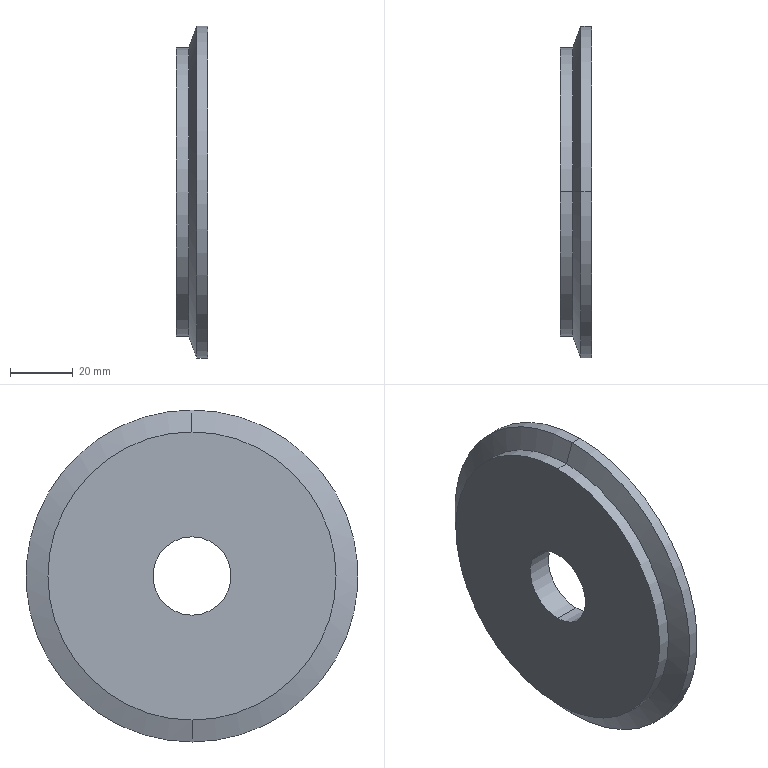Part | SolidWorks | features Revolution 1 | 1 solid | 13 faces | box 10 x 106 x 106 mm | volume 67420 mm3 | cylinder 8 | plane 3 | cone 2 | commonest cylinder face diameters 25 x2 62 x2 92 x2 106 x2
STEP:
#1=CARTESIAN_POINT('',(-7.771,0.,-46.));
#2=VERTEX_POINT('',#1);
#3=CARTESIAN_POINT('',(-7.771,0.,46.));
#4=VERTEX_POINT('',#3);
#5=CARTESIAN_POINT('',(-7.771,0.,0.));
#6=DIRECTION('',(1.,0.,0.));
#7=DIRECTION('',(0.,0.,-1.));
#8=AXIS2_PLACEMENT_3D('',#5,#6,#7);
#9=CIRCLE('',#8,46.);
#10=EDGE_CURVE('',#2,#4,#9,.T.);
#11=ORIENTED_EDGE('',*,*,#10,.T.);
#12=CARTESIAN_POINT('',(-5.271,0.,53.));
#13=VERTEX_POINT('',#12);
#14=CARTESIAN_POINT('',(-5.271,0.,53.));
#15=DIRECTION('',(0.3363,0.,0.9417));
#16=VECTOR('',#15,1000.);
#17=LINE('',#14,#16);
#18=EDGE_CURVE('',#4,#13,#17,.T.);
#19=ORIENTED_EDGE('',*,*,#18,.T.);
#20=CARTESIAN_POINT('',(-5.271,0.,-53.));
#21=VERTEX_POINT('',#20);
#22=CARTESIAN_POINT('',(-5.271,0.,0.));
#23=DIRECTION('',(1.,0.,0.));
#24=DIRECTION('',(0.,0.,-1.));
#25=AXIS2_PLACEMENT_3D('',#22,#23,#24);
#26=CIRCLE('',#25,53.);
#27=EDGE_CURVE('',#21,#13,#26,.T.);
#28=ORIENTED_EDGE('',*,*,#27,.F.);
#29=CARTESIAN_POINT('',(-5.271,0.,-53.));
#30=DIRECTION('',(0.3363,0.,-0.9417));
#31=VECTOR('',#30,1000.);
#32=LINE('',#29,#31);
#33=EDGE_CURVE('',#2,#21,#32,.T.);
#34=ORIENTED_EDGE('',*,*,#33,.F.);
#35=EDGE_LOOP('',(#11,#19,#28,#34));
#36=FACE_OUTER_BOUND('',#35,.T.);
#37=CARTESIAN_POINT('',(-5.271,0.,0.));
#38=DIRECTION('',(1.,0.,0.));
#39=DIRECTION('',(0.,0.,-1.));
#40=AXIS2_PLACEMENT_3D('',#37,#38,#39);
#41=CONICAL_SURFACE('',#40,53.,1.228);
#42=ADVANCED_FACE('',(#36),#41,.T.);
#43=ORIENTED_EDGE('',*,*,#27,.T.);
#44=CARTESIAN_POINT('',(-1.771,0.,53.));
#45=VERTEX_POINT('',#44);
#46=CARTESIAN_POINT('',(0.,0.,53.));
#47=DIRECTION('',(1.,0.,0.));
#48=VECTOR('',#47,1000.);
#49=LINE('',#46,#48);
#50=EDGE_CURVE('',#13,#45,#49,.T.);
#51=ORIENTED_EDGE('',*,*,#50,.T.);
#52=CARTESIAN_POINT('',(-1.771,0.,-53.));
#53=VERTEX_POINT('',#52);
#54=CARTESIAN_POINT('',(-1.771,0.,0.));
#55=DIRECTION('',(1.,0.,0.));
#56=DIRECTION('',(0.,0.,-1.));
#57=AXIS2_PLACEMENT_3D('',#54,#55,#56);
#58=CIRCLE('',#57,53.);
#59=EDGE_CURVE('',#53,#45,#58,.T.);
#60=ORIENTED_EDGE('',*,*,#59,.F.);
#61=CARTESIAN_POINT('',(0.,0.,-53.));
#62=DIRECTION('',(1.,0.,0.));
#63=VECTOR('',#62,1000.);
#64=LINE('',#61,#63);
#65=EDGE_CURVE('',#21,#53,#64,.T.);
#66=ORIENTED_EDGE('',*,*,#65,.F.);
#67=EDGE_LOOP('',(#43,#51,#60,#66));
#68=FACE_OUTER_BOUND('',#67,.T.);
#69=CARTESIAN_POINT('',(0.,0.,0.));
#70=DIRECTION('',(1.,0.,0.));
#71=DIRECTION('',(0.,0.,-1.));
#72=AXIS2_PLACEMENT_3D('',#69,#70,#71);
#73=CYLINDRICAL_SURFACE('',#72,53.);
#74=ADVANCED_FACE('',(#68),#73,.T.);
#75=CARTESIAN_POINT('',(-3.521,0.,31.));
#76=VERTEX_POINT('',#75);
#77=CARTESIAN_POINT('',(-3.521,0.,-31.));
#78=VERTEX_POINT('',#77);
#79=CARTESIAN_POINT('',(-3.521,0.,0.));
#80=DIRECTION('',(1.,0.,0.));
#81=DIRECTION('',(0.,0.,-1.));
#82=AXIS2_PLACEMENT_3D('',#79,#80,#81);
#83=CIRCLE('',#82,31.);
#84=EDGE_CURVE('',#76,#78,#83,.T.);
#85=ORIENTED_EDGE('',*,*,#84,.F.);
#86=CARTESIAN_POINT('',(-1.771,0.,31.));
#87=VERTEX_POINT('',#86);
#88=CARTESIAN_POINT('',(0.,0.,31.));
#89=DIRECTION('',(1.,0.,0.));
#90=VECTOR('',#89,1000.);
#91=LINE('',#88,#90);
#92=EDGE_CURVE('',#76,#87,#91,.T.);
#93=ORIENTED_EDGE('',*,*,#92,.T.);
#94=CARTESIAN_POINT('',(-1.771,0.,-31.));
#95=VERTEX_POINT('',#94);
#96=CARTESIAN_POINT('',(-1.771,0.,0.));
#97=DIRECTION('',(1.,0.,0.));
#98=DIRECTION('',(0.,0.,-1.));
#99=AXIS2_PLACEMENT_3D('',#96,#97,#98);
#100=CIRCLE('',#99,31.);
#101=EDGE_CURVE('',#87,#95,#100,.T.);
#102=ORIENTED_EDGE('',*,*,#101,.T.);
#103=CARTESIAN_POINT('',(0.,0.,-31.));
#104=DIRECTION('',(1.,0.,0.));
#105=VECTOR('',#104,1000.);
#106=LINE('',#103,#105);
#107=EDGE_CURVE('',#78,#95,#106,.T.);
#108=ORIENTED_EDGE('',*,*,#107,.F.);
#109=EDGE_LOOP('',(#85,#93,#102,#108));
#110=FACE_OUTER_BOUND('',#109,.T.);
#111=CARTESIAN_POINT('',(0.,0.,0.));
#112=DIRECTION('',(1.,0.,0.));
#113=DIRECTION('',(0.,0.,-1.));
#114=AXIS2_PLACEMENT_3D('',#111,#112,#113);
#115=CYLINDRICAL_SURFACE('',#114,31.);
#116=ADVANCED_FACE('',(#110),#115,.F.);
#117=CARTESIAN_POINT('',(-11.771,0.,12.5));
#118=VERTEX_POINT('',#117);
#119=CARTESIAN_POINT('',(-11.771,0.,-12.5));
#120=VERTEX_POINT('',#119);
#121=CARTESIAN_POINT('',(-11.771,0.,0.));
#122=DIRECTION('',(1.,0.,0.));
#123=DIRECTION('',(0.,0.,-1.));
#124=AXIS2_PLACEMENT_3D('',#121,#122,#123);
#125=CIRCLE('',#124,12.5);
#126=EDGE_CURVE('',#118,#120,#125,.T.);
#127=ORIENTED_EDGE('',*,*,#126,.F.);
#128=CARTESIAN_POINT('',(-3.521,0.,12.5));
#129=VERTEX_POINT('',#128);
#130=CARTESIAN_POINT('',(0.,0.,12.5));
#131=DIRECTION('',(1.,0.,0.));
#132=VECTOR('',#131,1000.);
#133=LINE('',#130,#132);
#134=EDGE_CURVE('',#118,#129,#133,.T.);
#135=ORIENTED_EDGE('',*,*,#134,.T.);
#136=CARTESIAN_POINT('',(-3.521,0.,-12.5));
#137=VERTEX_POINT('',#136);
#138=CARTESIAN_POINT('',(-3.521,0.,0.));
#139=DIRECTION('',(1.,0.,0.));
#140=DIRECTION('',(0.,0.,-1.));
#141=AXIS2_PLACEMENT_3D('',#138,#139,#140);
#142=CIRCLE('',#141,12.5);
#143=EDGE_CURVE('',#129,#137,#142,.T.);
#144=ORIENTED_EDGE('',*,*,#143,.T.);
#145=CARTESIAN_POINT('',(0.,0.,-12.5));
#146=DIRECTION('',(1.,0.,0.));
#147=VECTOR('',#146,1000.);
#148=LINE('',#145,#147);
#149=EDGE_CURVE('',#120,#137,#148,.T.);
#150=ORIENTED_EDGE('',*,*,#149,.F.);
#151=EDGE_LOOP('',(#127,#135,#144,#150));
#152=FACE_OUTER_BOUND('',#151,.T.);
#153=CARTESIAN_POINT('',(0.,0.,0.));
#154=DIRECTION('',(1.,0.,0.));
#155=DIRECTION('',(0.,0.,-1.));
#156=AXIS2_PLACEMENT_3D('',#153,#154,#155);
#157=CYLINDRICAL_SURFACE('',#156,12.5);
#158=ADVANCED_FACE('',(#152),#157,.F.);
#159=CARTESIAN_POINT('',(-11.771,0.,-46.));
#160=VERTEX_POINT('',#159);
#161=CARTESIAN_POINT('',(-11.771,0.,46.));
#162=VERTEX_POINT('',#161);
#163=CARTESIAN_POINT('',(-11.771,0.,0.));
#164=DIRECTION('',(1.,0.,0.));
#165=DIRECTION('',(0.,0.,-1.));
#166=AXIS2_PLACEMENT_3D('',#163,#164,#165);
#167=CIRCLE('',#166,46.);
#168=EDGE_CURVE('',#160,#162,#167,.T.);
#169=ORIENTED_EDGE('',*,*,#168,.T.);
#170=CARTESIAN_POINT('',(0.,0.,46.));
#171=DIRECTION('',(1.,0.,0.));
#172=VECTOR('',#171,1000.);
#173=LINE('',#170,#172);
#174=EDGE_CURVE('',#162,#4,#173,.T.);
#175=ORIENTED_EDGE('',*,*,#174,.T.);
#176=ORIENTED_EDGE('',*,*,#10,.F.);
#177=CARTESIAN_POINT('',(0.,0.,-46.));
#178=DIRECTION('',(1.,0.,0.));
#179=VECTOR('',#178,1000.);
#180=LINE('',#177,#179);
#181=EDGE_CURVE('',#160,#2,#180,.T.);
#182=ORIENTED_EDGE('',*,*,#181,.F.);
#183=EDGE_LOOP('',(#169,#175,#176,#182));
#184=FACE_OUTER_BOUND('',#183,.T.);
#185=CARTESIAN_POINT('',(0.,0.,0.));
#186=DIRECTION('',(1.,0.,0.));
#187=DIRECTION('',(0.,0.,-1.));
#188=AXIS2_PLACEMENT_3D('',#185,#186,#187);
#189=CYLINDRICAL_SURFACE('',#188,46.);
#190=ADVANCED_FACE('',(#184),#189,.T.);
#191=ORIENTED_EDGE('',*,*,#174,.F.);
#192=CARTESIAN_POINT('',(-11.771,0.,0.));
#193=DIRECTION('',(1.,0.,0.));
#194=DIRECTION('',(0.,0.,-1.));
#195=AXIS2_PLACEMENT_3D('',#192,#193,#194);
#196=CIRCLE('',#195,46.);
#197=EDGE_CURVE('',#162,#160,#196,.T.);
#198=ORIENTED_EDGE('',*,*,#197,.T.);
#199=ORIENTED_EDGE('',*,*,#181,.T.);
#200=CARTESIAN_POINT('',(-7.771,0.,0.));
#201=DIRECTION('',(1.,0.,0.));
#202=DIRECTION('',(0.,0.,-1.));
#203=AXIS2_PLACEMENT_3D('',#200,#201,#202);
#204=CIRCLE('',#203,46.);
#205=EDGE_CURVE('',#4,#2,#204,.T.);
#206=ORIENTED_EDGE('',*,*,#205,.F.);
#207=EDGE_LOOP('',(#191,#198,#199,#206));
#208=FACE_OUTER_BOUND('',#207,.T.);
#209=CARTESIAN_POINT('',(0.,0.,0.));
#210=DIRECTION('',(1.,0.,0.));
#211=DIRECTION('',(0.,0.,-1.));
#212=AXIS2_PLACEMENT_3D('',#209,#210,#211);
#213=CYLINDRICAL_SURFACE('',#212,46.);
#214=ADVANCED_FACE('',(#208),#213,.T.);
#215=CARTESIAN_POINT('',(-11.771,0.,0.));
#216=DIRECTION('',(1.,0.,0.));
#217=DIRECTION('',(0.,0.,-1.));
#218=AXIS2_PLACEMENT_3D('',#215,#216,#217);
#219=CIRCLE('',#218,12.5);
#220=EDGE_CURVE('',#120,#118,#219,.T.);
#221=ORIENTED_EDGE('',*,*,#220,.T.);
#222=ORIENTED_EDGE('',*,*,#126,.T.);
#223=EDGE_LOOP('',(#221,#222));
#224=FACE_BOUND('',#223,.T.);
#225=ORIENTED_EDGE('',*,*,#168,.F.);
#226=ORIENTED_EDGE('',*,*,#197,.F.);
#227=EDGE_LOOP('',(#225,#226));
#228=FACE_OUTER_BOUND('',#227,.T.);
#229=CARTESIAN_POINT('',(-11.771,46.,0.));
#230=DIRECTION('',(-1.,0.,0.));
#231=DIRECTION('',(0.,0.,1.));
#232=AXIS2_PLACEMENT_3D('',#229,#230,#231);
#233=PLANE('',#232);
#234=ADVANCED_FACE('',(#224,#228),#233,.T.);
#235=ORIENTED_EDGE('',*,*,#134,.F.);
#236=ORIENTED_EDGE('',*,*,#220,.F.);
#237=ORIENTED_EDGE('',*,*,#149,.T.);
#238=CARTESIAN_POINT('',(-3.521,0.,0.));
#239=DIRECTION('',(1.,0.,0.));
#240=DIRECTION('',(0.,0.,-1.));
#241=AXIS2_PLACEMENT_3D('',#238,#239,#240);
#242=CIRCLE('',#241,12.5);
#243=EDGE_CURVE('',#137,#129,#242,.T.);
#244=ORIENTED_EDGE('',*,*,#243,.T.);
#245=EDGE_LOOP('',(#235,#236,#237,#244));
#246=FACE_OUTER_BOUND('',#245,.T.);
#247=CARTESIAN_POINT('',(0.,0.,0.));
#248=DIRECTION('',(1.,0.,0.));
#249=DIRECTION('',(0.,0.,-1.));
#250=AXIS2_PLACEMENT_3D('',#247,#248,#249);
#251=CYLINDRICAL_SURFACE('',#250,12.5);
#252=ADVANCED_FACE('',(#246),#251,.F.);
#253=CARTESIAN_POINT('',(-3.521,0.,0.));
#254=DIRECTION('',(1.,0.,0.));
#255=DIRECTION('',(0.,0.,-1.));
#256=AXIS2_PLACEMENT_3D('',#253,#254,#255);
#257=CIRCLE('',#256,31.);
#258=EDGE_CURVE('',#78,#76,#257,.T.);
#259=ORIENTED_EDGE('',*,*,#258,.T.);
#260=ORIENTED_EDGE('',*,*,#84,.T.);
#261=EDGE_LOOP('',(#259,#260));
#262=FACE_OUTER_BOUND('',#261,.T.);
#263=ORIENTED_EDGE('',*,*,#243,.F.);
#264=ORIENTED_EDGE('',*,*,#143,.F.);
#265=EDGE_LOOP('',(#263,#264));
#266=FACE_BOUND('',#265,.T.);
#267=CARTESIAN_POINT('',(-3.521,12.5,0.));
#268=DIRECTION('',(1.,0.,0.));
#269=DIRECTION('',(0.,0.,-1.));
#270=AXIS2_PLACEMENT_3D('',#267,#268,#269);
#271=PLANE('',#270);
#272=ADVANCED_FACE('',(#262,#266),#271,.T.);
#273=ORIENTED_EDGE('',*,*,#92,.F.);
#274=ORIENTED_EDGE('',*,*,#258,.F.);
#275=ORIENTED_EDGE('',*,*,#107,.T.);
#276=CARTESIAN_POINT('',(-1.771,0.,0.));
#277=DIRECTION('',(1.,0.,0.));
#278=DIRECTION('',(0.,0.,-1.));
#279=AXIS2_PLACEMENT_3D('',#276,#277,#278);
#280=CIRCLE('',#279,31.);
#281=EDGE_CURVE('',#95,#87,#280,.T.);
#282=ORIENTED_EDGE('',*,*,#281,.T.);
#283=EDGE_LOOP('',(#273,#274,#275,#282));
#284=FACE_OUTER_BOUND('',#283,.T.);
#285=CARTESIAN_POINT('',(0.,0.,0.));
#286=DIRECTION('',(1.,0.,0.));
#287=DIRECTION('',(0.,0.,-1.));
#288=AXIS2_PLACEMENT_3D('',#285,#286,#287);
#289=CYLINDRICAL_SURFACE('',#288,31.);
#290=ADVANCED_FACE('',(#284),#289,.F.);
#291=ORIENTED_EDGE('',*,*,#59,.T.);
#292=CARTESIAN_POINT('',(-1.771,0.,0.));
#293=DIRECTION('',(1.,0.,0.));
#294=DIRECTION('',(0.,0.,-1.));
#295=AXIS2_PLACEMENT_3D('',#292,#293,#294);
#296=CIRCLE('',#295,53.);
#297=EDGE_CURVE('',#45,#53,#296,.T.);
#298=ORIENTED_EDGE('',*,*,#297,.T.);
#299=EDGE_LOOP('',(#291,#298));
#300=FACE_OUTER_BOUND('',#299,.T.);
#301=ORIENTED_EDGE('',*,*,#281,.F.);
#302=ORIENTED_EDGE('',*,*,#101,.F.);
#303=EDGE_LOOP('',(#301,#302));
#304=FACE_BOUND('',#303,.T.);
#305=CARTESIAN_POINT('',(-1.771,31.,0.));
#306=DIRECTION('',(1.,0.,0.));
#307=DIRECTION('',(0.,0.,-1.));
#308=AXIS2_PLACEMENT_3D('',#305,#306,#307);
#309=PLANE('',#308);
#310=ADVANCED_FACE('',(#300,#304),#309,.T.);
#311=ORIENTED_EDGE('',*,*,#50,.F.);
#312=CARTESIAN_POINT('',(-5.271,0.,0.));
#313=DIRECTION('',(1.,0.,0.));
#314=DIRECTION('',(0.,0.,-1.));
#315=AXIS2_PLACEMENT_3D('',#312,#313,#314);
#316=CIRCLE('',#315,53.);
#317=EDGE_CURVE('',#13,#21,#316,.T.);
#318=ORIENTED_EDGE('',*,*,#317,.T.);
#319=ORIENTED_EDGE('',*,*,#65,.T.);
#320=ORIENTED_EDGE('',*,*,#297,.F.);
#321=EDGE_LOOP('',(#311,#318,#319,#320));
#322=FACE_OUTER_BOUND('',#321,.T.);
#323=CARTESIAN_POINT('',(0.,0.,0.));
#324=DIRECTION('',(1.,0.,0.));
#325=DIRECTION('',(0.,0.,-1.));
#326=AXIS2_PLACEMENT_3D('',#323,#324,#325);
#327=CYLINDRICAL_SURFACE('',#326,53.);
#328=ADVANCED_FACE('',(#322),#327,.T.);
#329=ORIENTED_EDGE('',*,*,#18,.F.);
#330=ORIENTED_EDGE('',*,*,#205,.T.);
#331=ORIENTED_EDGE('',*,*,#33,.T.);
#332=ORIENTED_EDGE('',*,*,#317,.F.);
#333=EDGE_LOOP('',(#329,#330,#331,#332));
#334=FACE_OUTER_BOUND('',#333,.T.);
#335=CARTESIAN_POINT('',(-5.271,0.,0.));
#336=DIRECTION('',(1.,0.,0.));
#337=DIRECTION('',(0.,0.,-1.));
#338=AXIS2_PLACEMENT_3D('',#335,#336,#337);
#339=CONICAL_SURFACE('',#338,53.,1.228);
#340=ADVANCED_FACE('',(#334),#339,.T.);
#341=CLOSED_SHELL('',(#42,#74,#116,#158,#190,#214,#234,#252,#272,#290,#310,#328,#340));
#342=MANIFOLD_SOLID_BREP('',#341);
#343=CARTESIAN_POINT('',(0.,0.,0.));
#344=DIRECTION('',(0.,0.,1.));
#345=DIRECTION('',(1.,0.,0.));
#346=AXIS2_PLACEMENT_3D('',#343,#344,#345);
#347=(LENGTH_UNIT()NAMED_UNIT(*)SI_UNIT(.MILLI.,.METRE.));
#348=UNCERTAINTY_MEASURE_WITH_UNIT(LENGTH_MEASURE(0.00001),#347,'','');
#349=(NAMED_UNIT(*)PLANE_ANGLE_UNIT()SI_UNIT($,.RADIAN.));
#350=(NAMED_UNIT(*)SI_UNIT($,.STERADIAN.)SOLID_ANGLE_UNIT());
#351=(GEOMETRIC_REPRESENTATION_CONTEXT(3)GLOBAL_UNCERTAINTY_ASSIGNED_CONTEXT((#348))GLOBAL_UNIT_ASSIGNED_CONTEXT((#347,#349,#350))REPRESENTATION_CONTEXT('',''));
#352=ADVANCED_BREP_SHAPE_REPRESENTATION('',(#342,#346),#351);